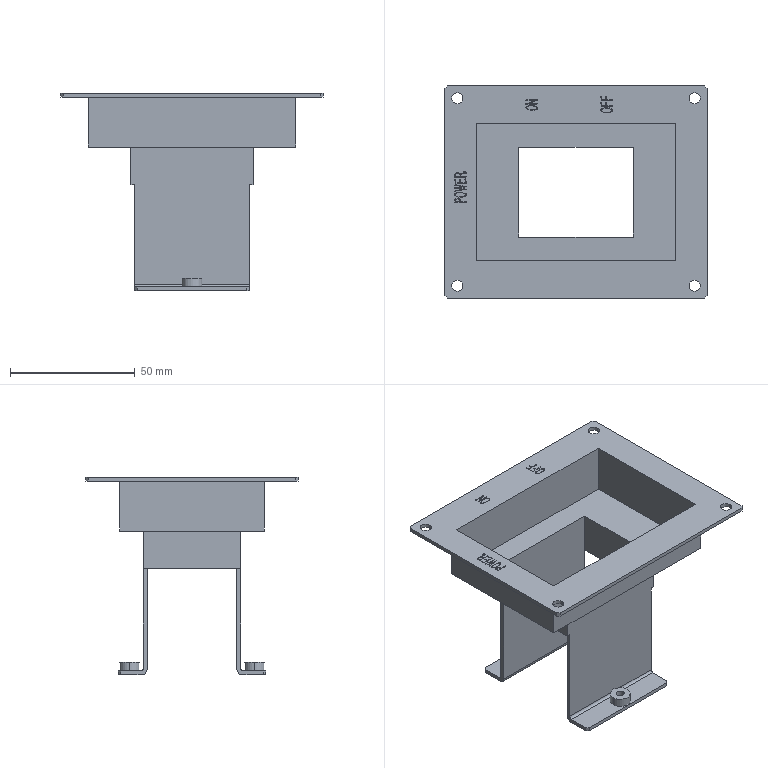Part | STEP file | 电源1 | 1 solid | 293 faces | box 105 x 85 x 79 mm | volume 30351 mm3 | plane 179 | spline 94 | cylinder 20 | commonest cylinder face diameters 4.5 x8 3.242 x4 8 x4 2 x2 4 x2